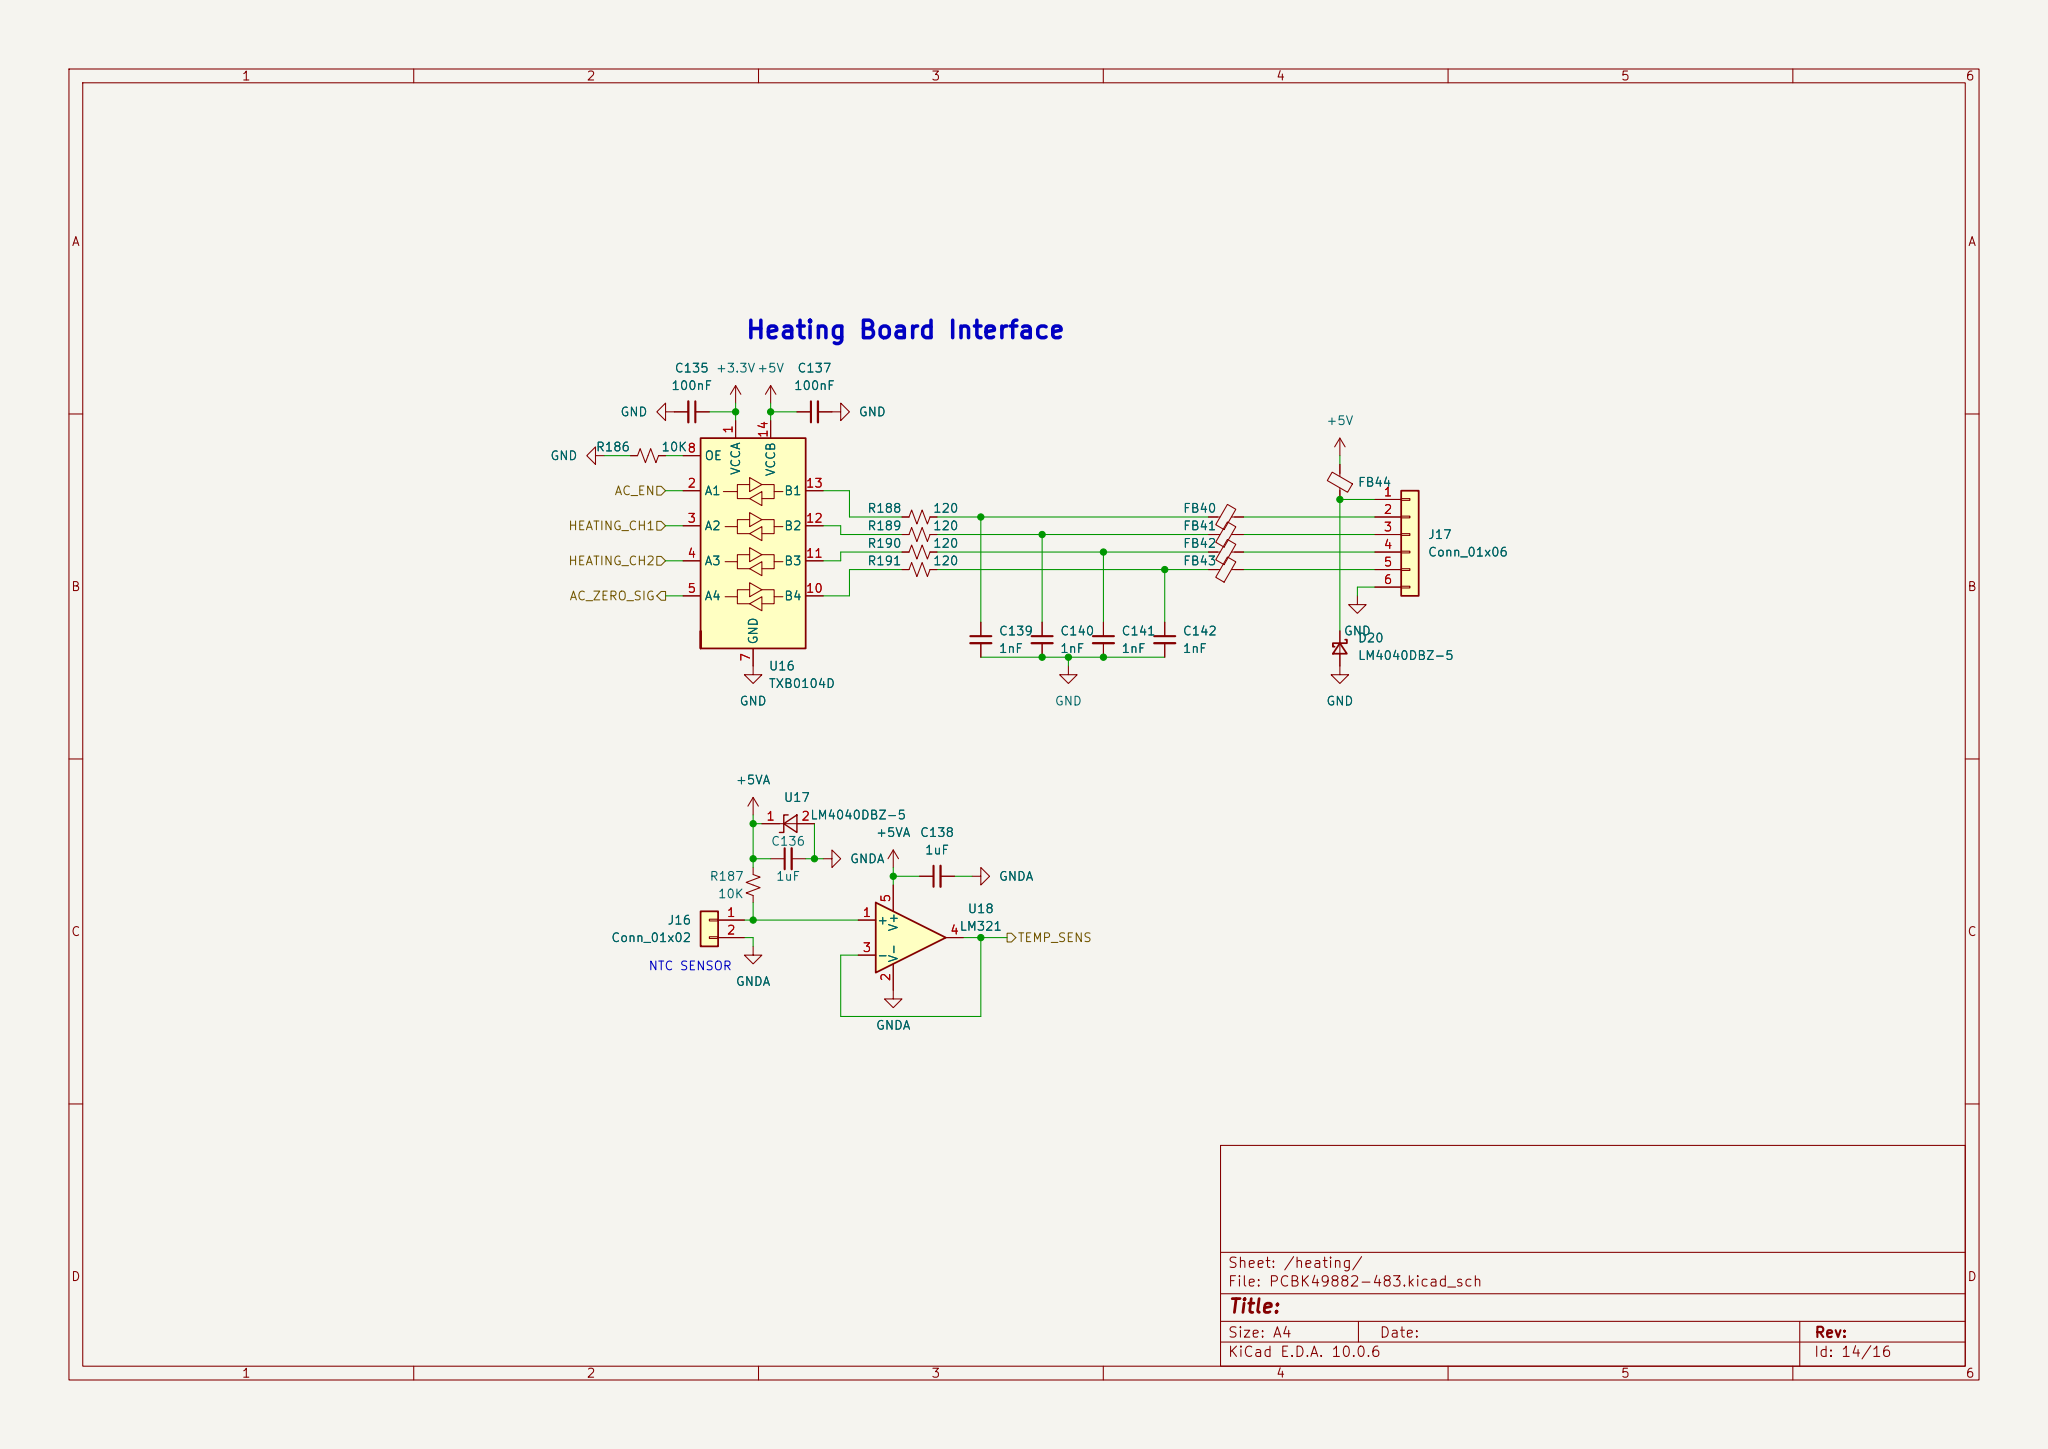Circuit board | KiCad | 536 parts | 438 nets | one sheet of the schematic
Parts on this sheet (reference | value | footprint):
C135
C136 | 1uF | Capacitor_SMD:C_0603_1608Metric
C137 | 100nF | Capacitor_SMD:C_0603_1608Metric
C138 | 1uF | Capacitor_SMD:C_0603_1608Metric
C139
C140
C141
C142
D20 | LM4040DBZ-5 | Package_TO_SOT_SMD:SOT-23
FB40
FB41
FB42
FB43
FB44 | FerriteBead_Small | Inductor_SMD:L_0805_2012Metric
J16 | Conn_01x02 | Connector_Molex:Molex_MicroClasp_55932-0230_1x02_P2.00mm_Vertical
J17 | Conn_01x06 | Connector_Molex:Molex_MicroClasp_55932-0630_1x06_P2.00mm_Vertical
R186 | 10K | Resistor_SMD:R_0603_1608Metric
R187 | 10K | Resistor_SMD:R_0603_1608Metric
R188
R189
R190
R191
U16 | TXB0104D | Package_SO:SOIC-14_3.9x8.7mm_P1.27mm
U17 | LM4040DBZ-5 | Package_TO_SOT_SMD:SOT-23
U18 | LM321 | Package_TO_SOT_SMD:SOT-23-5
Nets of these parts (net: part-pin ...):
+3.3V: C135-1 U16-1
+5V: C137-1 FB44-2 U16-14
+5VA: C136-1 C138-1 R187-1 U17-1 U18-5
/core_board_b2b/PC6{slash}HEATING_CH1: U16-3
/core_board_b2b/PC7{slash}HEATING_CH2: U16-4
/core_board_b2b/PD3{slash}AC_EN: U16-2
/core_board_b2b/PD4{slash}AC_ZERO_SIG: U16-5
/sensors/CH10: U18-3 U18-4
GND: C135-2 C137-2 C139-2 C140-2 C141-2 C142-2 D20-2 J17-6 R186-1 U16-7
GNDA: C136-2 C138-2 J16-2 U17-2 U18-2
Net-(C139-Pad1): C139-1 FB40-1 R188-2
Net-(C140-Pad1): C140-1 FB41-1 R189-2
Net-(C141-Pad1): C141-1 FB42-1 R190-2
Net-(C142-Pad1): C142-1 FB43-1 R191-2
Net-(D20-K): D20-1 FB44-1 J17-1
Net-(J16-Pin_1): J16-1 R187-2 U18-1
Net-(J17-Pin_2): FB40-2 J17-2
Net-(J17-Pin_3): FB41-2 J17-3
Net-(J17-Pin_4): FB42-2 J17-4
Net-(J17-Pin_5): FB43-2 J17-5
Net-(U16-B1): R188-1 U16-13
Net-(U16-B2): R189-1 U16-12
Net-(U16-B3): R190-1 U16-11
Net-(U16-B4): R191-1 U16-10
Net-(U16-OE): R186-2 U16-8
unconnected-(U16-NC-Pad6): U16-6
unconnected-(U16-NC-Pad9): U16-9